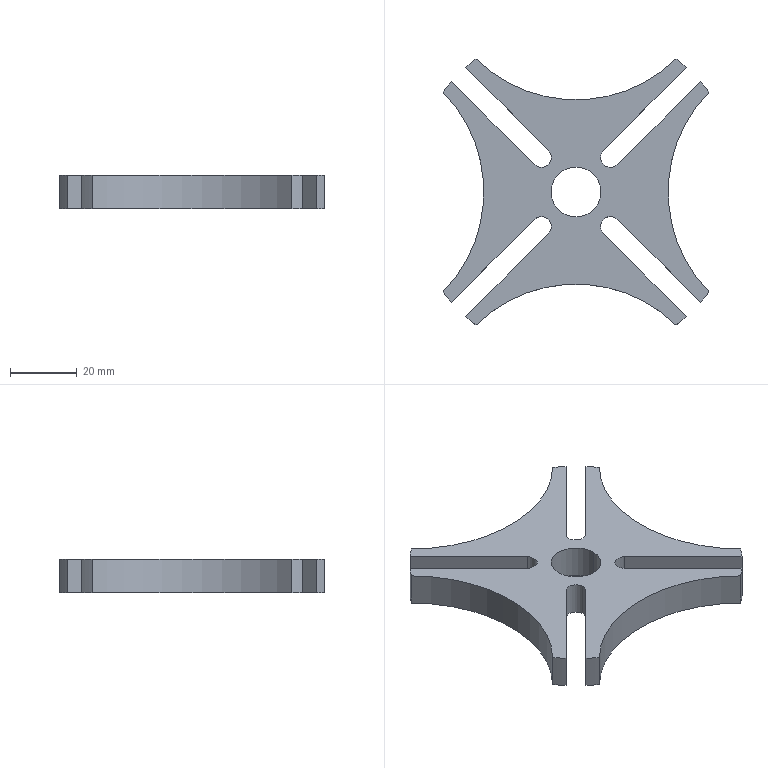Part | STEP file | 1 solid | 30 faces | box 79.917 x 79.917 x 10 mm | volume 31022 mm3 | cylinder 20 | plane 10 | commonest cylinder face diameters 100 x8 6 x6 86 x4 15 x2